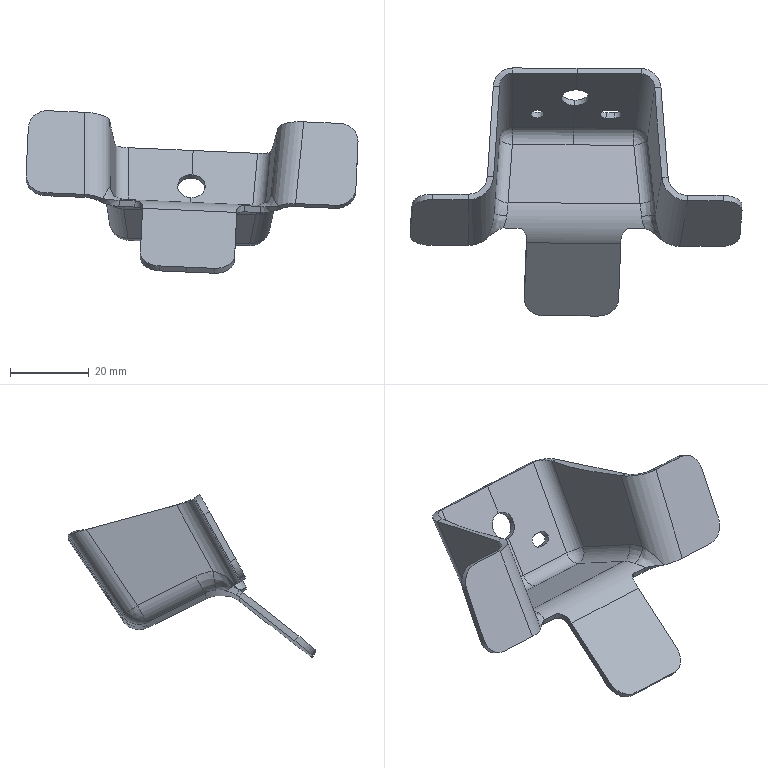Part | STEP file | FNA5401591 | 1 solid | 90 faces | box 84.51 x 63.094 x 41.379 mm | volume 7895 mm3 | spline 55 | cylinder 18 | plane 12 | sphere 4 | other 1 | commonest cylinder face diameters 10 x8 6.8 x6 13.2 x2 16 x1 19.2 x1